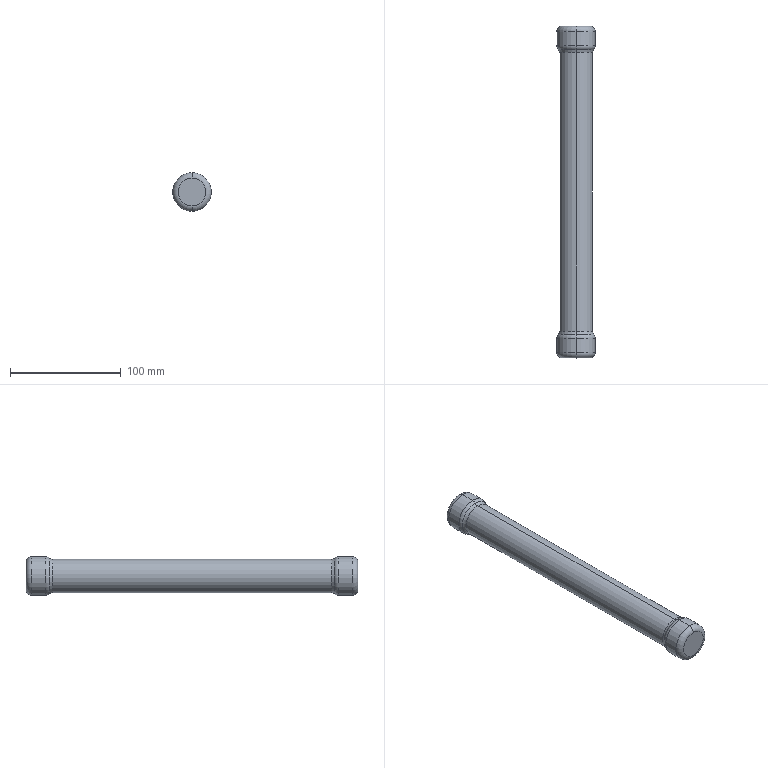Part | SolidWorks | features Fillet 3, Extrusion 1, ICE 1, MirrorPattern 1 | 1 solid | 20 faces | box 35 x 300 x 35 mm | volume 221656 mm3 | torus 12 | cylinder 6 | plane 2 | commonest cylinder face diameters 35 x4 30 x2
STEP:
#1=CARTESIAN_POINT('',(0.,132.284,17.5));
#2=VERTEX_POINT('',#1);
#3=CARTESIAN_POINT('',(0.,132.284,-17.5));
#4=VERTEX_POINT('',#3);
#5=CARTESIAN_POINT('',(0.,132.284,0.));
#6=DIRECTION('',(0.,1.,0.));
#7=DIRECTION('',(0.,0.,-1.));
#8=AXIS2_PLACEMENT_3D('',#5,#6,#7);
#9=CIRCLE('',#8,17.5);
#10=EDGE_CURVE('',#2,#4,#9,.T.);
#11=ORIENTED_EDGE('',*,*,#10,.F.);
#12=CARTESIAN_POINT('',(0.,128.977,16.25));
#13=VERTEX_POINT('',#12);
#14=CARTESIAN_POINT('',(0.,132.284,12.5));
#15=DIRECTION('',(1.,0.,0.));
#16=DIRECTION('',(0.,0.,-1.));
#17=AXIS2_PLACEMENT_3D('',#14,#15,#16);
#18=CIRCLE('',#17,5.);
#19=EDGE_CURVE('',#2,#13,#18,.T.);
#20=ORIENTED_EDGE('',*,*,#19,.T.);
#21=CARTESIAN_POINT('',(0.,128.977,-16.25));
#22=VERTEX_POINT('',#21);
#23=CARTESIAN_POINT('',(0.,128.977,0.));
#24=DIRECTION('',(0.,-1.,0.));
#25=DIRECTION('',(0.,0.,-1.));
#26=AXIS2_PLACEMENT_3D('',#23,#24,#25);
#27=CIRCLE('',#26,16.25);
#28=EDGE_CURVE('',#22,#13,#27,.T.);
#29=ORIENTED_EDGE('',*,*,#28,.F.);
#30=CARTESIAN_POINT('',(0.,132.284,-12.5));
#31=DIRECTION('',(-1.,0.,0.));
#32=DIRECTION('',(0.,0.,1.));
#33=AXIS2_PLACEMENT_3D('',#30,#31,#32);
#34=CIRCLE('',#33,5.);
#35=EDGE_CURVE('',#4,#22,#34,.T.);
#36=ORIENTED_EDGE('',*,*,#35,.F.);
#37=EDGE_LOOP('',(#11,#20,#29,#36));
#38=FACE_OUTER_BOUND('',#37,.T.);
#39=CARTESIAN_POINT('',(0.,132.284,0.));
#40=DIRECTION('',(0.,-1.,0.));
#41=DIRECTION('',(0.,0.,-1.));
#42=AXIS2_PLACEMENT_3D('',#39,#40,#41);
#43=TOROIDAL_SURFACE('',#42,12.5,5.);
#44=ADVANCED_FACE('',(#38),#43,.T.);
#45=CARTESIAN_POINT('',(0.,-128.977,16.25));
#46=VERTEX_POINT('',#45);
#47=CARTESIAN_POINT('',(0.,-128.977,-16.25));
#48=VERTEX_POINT('',#47);
#49=CARTESIAN_POINT('',(0.,-128.977,0.));
#50=DIRECTION('',(0.,1.,0.));
#51=DIRECTION('',(0.,0.,1.));
#52=AXIS2_PLACEMENT_3D('',#49,#50,#51);
#53=CIRCLE('',#52,16.25);
#54=EDGE_CURVE('',#46,#48,#53,.T.);
#55=ORIENTED_EDGE('',*,*,#54,.F.);
#56=CARTESIAN_POINT('',(0.,-132.284,17.5));
#57=VERTEX_POINT('',#56);
#58=CARTESIAN_POINT('',(0.,-132.284,12.5));
#59=DIRECTION('',(1.,0.,0.));
#60=DIRECTION('',(0.,0.,-1.));
#61=AXIS2_PLACEMENT_3D('',#58,#59,#60);
#62=CIRCLE('',#61,5.);
#63=EDGE_CURVE('',#46,#57,#62,.T.);
#64=ORIENTED_EDGE('',*,*,#63,.T.);
#65=CARTESIAN_POINT('',(0.,-132.284,-17.5));
#66=VERTEX_POINT('',#65);
#67=CARTESIAN_POINT('',(0.,-132.284,0.));
#68=DIRECTION('',(0.,-1.,0.));
#69=DIRECTION('',(0.,0.,-1.));
#70=AXIS2_PLACEMENT_3D('',#67,#68,#69);
#71=CIRCLE('',#70,17.5);
#72=EDGE_CURVE('',#66,#57,#71,.T.);
#73=ORIENTED_EDGE('',*,*,#72,.F.);
#74=CARTESIAN_POINT('',(0.,-132.284,-12.5));
#75=DIRECTION('',(-1.,0.,0.));
#76=DIRECTION('',(0.,0.,1.));
#77=AXIS2_PLACEMENT_3D('',#74,#75,#76);
#78=CIRCLE('',#77,5.);
#79=EDGE_CURVE('',#48,#66,#78,.T.);
#80=ORIENTED_EDGE('',*,*,#79,.F.);
#81=EDGE_LOOP('',(#55,#64,#73,#80));
#82=FACE_OUTER_BOUND('',#81,.T.);
#83=CARTESIAN_POINT('',(0.,-132.284,0.));
#84=DIRECTION('',(0.,-1.,0.));
#85=DIRECTION('',(0.,0.,-1.));
#86=AXIS2_PLACEMENT_3D('',#83,#84,#85);
#87=TOROIDAL_SURFACE('',#86,12.5,5.);
#88=ADVANCED_FACE('',(#82),#87,.T.);
#89=CARTESIAN_POINT('',(0.,-145.,17.5));
#90=VERTEX_POINT('',#89);
#91=CARTESIAN_POINT('',(0.,-145.,-17.5));
#92=VERTEX_POINT('',#91);
#93=CARTESIAN_POINT('',(0.,-145.,0.));
#94=DIRECTION('',(0.,1.,0.));
#95=DIRECTION('',(0.,0.,-1.));
#96=AXIS2_PLACEMENT_3D('',#93,#94,#95);
#97=CIRCLE('',#96,17.5);
#98=EDGE_CURVE('',#90,#92,#97,.T.);
#99=ORIENTED_EDGE('',*,*,#98,.F.);
#100=CARTESIAN_POINT('',(0.,-150.,12.5));
#101=VERTEX_POINT('',#100);
#102=CARTESIAN_POINT('',(0.,-145.,12.5));
#103=DIRECTION('',(1.,0.,0.));
#104=DIRECTION('',(0.,0.,-1.));
#105=AXIS2_PLACEMENT_3D('',#102,#103,#104);
#106=CIRCLE('',#105,5.);
#107=EDGE_CURVE('',#90,#101,#106,.T.);
#108=ORIENTED_EDGE('',*,*,#107,.T.);
#109=CARTESIAN_POINT('',(0.,-150.,-12.5));
#110=VERTEX_POINT('',#109);
#111=CARTESIAN_POINT('',(0.,-150.,0.));
#112=DIRECTION('',(0.,-1.,0.));
#113=DIRECTION('',(0.,0.,-1.));
#114=AXIS2_PLACEMENT_3D('',#111,#112,#113);
#115=CIRCLE('',#114,12.5);
#116=EDGE_CURVE('',#110,#101,#115,.T.);
#117=ORIENTED_EDGE('',*,*,#116,.F.);
#118=CARTESIAN_POINT('',(0.,-145.,-12.5));
#119=DIRECTION('',(-1.,0.,0.));
#120=DIRECTION('',(0.,0.,1.));
#121=AXIS2_PLACEMENT_3D('',#118,#119,#120);
#122=CIRCLE('',#121,5.);
#123=EDGE_CURVE('',#92,#110,#122,.T.);
#124=ORIENTED_EDGE('',*,*,#123,.F.);
#125=EDGE_LOOP('',(#99,#108,#117,#124));
#126=FACE_OUTER_BOUND('',#125,.T.);
#127=CARTESIAN_POINT('',(0.,-145.,0.));
#128=DIRECTION('',(0.,-1.,0.));
#129=DIRECTION('',(0.,0.,-1.));
#130=AXIS2_PLACEMENT_3D('',#127,#128,#129);
#131=TOROIDAL_SURFACE('',#130,12.5,5.);
#132=ADVANCED_FACE('',(#126),#131,.T.);
#133=CARTESIAN_POINT('',(0.,145.,-17.5));
#134=VERTEX_POINT('',#133);
#135=CARTESIAN_POINT('',(0.,145.,17.5));
#136=VERTEX_POINT('',#135);
#137=CARTESIAN_POINT('',(0.,145.,0.));
#138=DIRECTION('',(0.,-1.,0.));
#139=DIRECTION('',(0.,0.,1.));
#140=AXIS2_PLACEMENT_3D('',#137,#138,#139);
#141=CIRCLE('',#140,17.5);
#142=EDGE_CURVE('',#134,#136,#141,.T.);
#143=ORIENTED_EDGE('',*,*,#142,.F.);
#144=CARTESIAN_POINT('',(0.,150.,-12.5));
#145=VERTEX_POINT('',#144);
#146=CARTESIAN_POINT('',(0.,145.,-12.5));
#147=DIRECTION('',(1.,0.,0.));
#148=DIRECTION('',(0.,0.,-1.));
#149=AXIS2_PLACEMENT_3D('',#146,#147,#148);
#150=CIRCLE('',#149,5.);
#151=EDGE_CURVE('',#134,#145,#150,.T.);
#152=ORIENTED_EDGE('',*,*,#151,.T.);
#153=CARTESIAN_POINT('',(0.,150.,12.5));
#154=VERTEX_POINT('',#153);
#155=CARTESIAN_POINT('',(0.,150.,0.));
#156=DIRECTION('',(0.,1.,0.));
#157=DIRECTION('',(0.,0.,1.));
#158=AXIS2_PLACEMENT_3D('',#155,#156,#157);
#159=CIRCLE('',#158,12.5);
#160=EDGE_CURVE('',#154,#145,#159,.T.);
#161=ORIENTED_EDGE('',*,*,#160,.F.);
#162=CARTESIAN_POINT('',(0.,145.,12.5));
#163=DIRECTION('',(-1.,0.,0.));
#164=DIRECTION('',(0.,0.,1.));
#165=AXIS2_PLACEMENT_3D('',#162,#163,#164);
#166=CIRCLE('',#165,5.);
#167=EDGE_CURVE('',#136,#154,#166,.T.);
#168=ORIENTED_EDGE('',*,*,#167,.F.);
#169=EDGE_LOOP('',(#143,#152,#161,#168));
#170=FACE_OUTER_BOUND('',#169,.T.);
#171=CARTESIAN_POINT('',(0.,145.,0.));
#172=DIRECTION('',(0.,1.,0.));
#173=DIRECTION('',(0.,0.,1.));
#174=AXIS2_PLACEMENT_3D('',#171,#172,#173);
#175=TOROIDAL_SURFACE('',#174,12.5,5.);
#176=ADVANCED_FACE('',(#170),#175,.T.);
#177=CARTESIAN_POINT('',(0.,-128.977,0.));
#178=DIRECTION('',(0.,1.,0.));
#179=DIRECTION('',(0.,0.,1.));
#180=AXIS2_PLACEMENT_3D('',#177,#178,#179);
#181=CIRCLE('',#180,16.25);
#182=EDGE_CURVE('',#48,#46,#181,.T.);
#183=ORIENTED_EDGE('',*,*,#182,.T.);
#184=CARTESIAN_POINT('',(0.,-125.67,15.));
#185=VERTEX_POINT('',#184);
#186=CARTESIAN_POINT('',(0.,-125.67,20.));
#187=DIRECTION('',(1.,0.,0.));
#188=DIRECTION('',(0.,0.,-1.));
#189=AXIS2_PLACEMENT_3D('',#186,#187,#188);
#190=CIRCLE('',#189,5.);
#191=EDGE_CURVE('',#46,#185,#190,.T.);
#192=ORIENTED_EDGE('',*,*,#191,.T.);
#193=CARTESIAN_POINT('',(0.,-125.67,-15.));
#194=VERTEX_POINT('',#193);
#195=CARTESIAN_POINT('',(0.,-125.67,0.));
#196=DIRECTION('',(0.,1.,0.));
#197=DIRECTION('',(0.,0.,-1.));
#198=AXIS2_PLACEMENT_3D('',#195,#196,#197);
#199=CIRCLE('',#198,15.);
#200=EDGE_CURVE('',#194,#185,#199,.T.);
#201=ORIENTED_EDGE('',*,*,#200,.F.);
#202=CARTESIAN_POINT('',(0.,-125.67,-20.));
#203=DIRECTION('',(-1.,0.,0.));
#204=DIRECTION('',(0.,0.,1.));
#205=AXIS2_PLACEMENT_3D('',#202,#203,#204);
#206=CIRCLE('',#205,5.);
#207=EDGE_CURVE('',#48,#194,#206,.T.);
#208=ORIENTED_EDGE('',*,*,#207,.F.);
#209=EDGE_LOOP('',(#183,#192,#201,#208));
#210=FACE_OUTER_BOUND('',#209,.T.);
#211=CARTESIAN_POINT('',(0.,-125.67,0.));
#212=DIRECTION('',(0.,-1.,0.));
#213=DIRECTION('',(0.,0.,-1.));
#214=AXIS2_PLACEMENT_3D('',#211,#212,#213);
#215=TOROIDAL_SURFACE('',#214,20.,5.);
#216=ADVANCED_FACE('',(#210),#215,.F.);
#217=CARTESIAN_POINT('',(0.,128.977,0.));
#218=DIRECTION('',(0.,-1.,0.));
#219=DIRECTION('',(0.,0.,-1.));
#220=AXIS2_PLACEMENT_3D('',#217,#218,#219);
#221=CIRCLE('',#220,16.25);
#222=EDGE_CURVE('',#13,#22,#221,.T.);
#223=ORIENTED_EDGE('',*,*,#222,.T.);
#224=CARTESIAN_POINT('',(0.,125.67,-15.));
#225=VERTEX_POINT('',#224);
#226=CARTESIAN_POINT('',(0.,125.67,-20.));
#227=DIRECTION('',(1.,0.,0.));
#228=DIRECTION('',(0.,0.,-1.));
#229=AXIS2_PLACEMENT_3D('',#226,#227,#228);
#230=CIRCLE('',#229,5.);
#231=EDGE_CURVE('',#22,#225,#230,.T.);
#232=ORIENTED_EDGE('',*,*,#231,.T.);
#233=CARTESIAN_POINT('',(0.,125.67,15.));
#234=VERTEX_POINT('',#233);
#235=CARTESIAN_POINT('',(0.,125.67,0.));
#236=DIRECTION('',(0.,-1.,0.));
#237=DIRECTION('',(0.,0.,1.));
#238=AXIS2_PLACEMENT_3D('',#235,#236,#237);
#239=CIRCLE('',#238,15.);
#240=EDGE_CURVE('',#234,#225,#239,.T.);
#241=ORIENTED_EDGE('',*,*,#240,.F.);
#242=CARTESIAN_POINT('',(0.,125.67,20.));
#243=DIRECTION('',(-1.,0.,0.));
#244=DIRECTION('',(0.,0.,1.));
#245=AXIS2_PLACEMENT_3D('',#242,#243,#244);
#246=CIRCLE('',#245,5.);
#247=EDGE_CURVE('',#13,#234,#246,.T.);
#248=ORIENTED_EDGE('',*,*,#247,.F.);
#249=EDGE_LOOP('',(#223,#232,#241,#248));
#250=FACE_OUTER_BOUND('',#249,.T.);
#251=CARTESIAN_POINT('',(0.,125.67,0.));
#252=DIRECTION('',(0.,1.,0.));
#253=DIRECTION('',(0.,0.,1.));
#254=AXIS2_PLACEMENT_3D('',#251,#252,#253);
#255=TOROIDAL_SURFACE('',#254,20.,5.);
#256=ADVANCED_FACE('',(#250),#255,.F.);
#257=ORIENTED_EDGE('',*,*,#98,.T.);
#258=CARTESIAN_POINT('',(0.,-150.,-17.5));
#259=DIRECTION('',(0.,1.,0.));
#260=VECTOR('',#259,1000.);
#261=LINE('',#258,#260);
#262=EDGE_CURVE('',#92,#66,#261,.T.);
#263=ORIENTED_EDGE('',*,*,#262,.T.);
#264=ORIENTED_EDGE('',*,*,#72,.T.);
#265=CARTESIAN_POINT('',(0.,-150.,17.5));
#266=DIRECTION('',(0.,1.,0.));
#267=VECTOR('',#266,1000.);
#268=LINE('',#265,#267);
#269=EDGE_CURVE('',#90,#57,#268,.T.);
#270=ORIENTED_EDGE('',*,*,#269,.F.);
#271=EDGE_LOOP('',(#257,#263,#264,#270));
#272=FACE_OUTER_BOUND('',#271,.T.);
#273=CARTESIAN_POINT('',(0.,-150.,0.));
#274=DIRECTION('',(0.,1.,0.));
#275=DIRECTION('',(0.,0.,1.));
#276=AXIS2_PLACEMENT_3D('',#273,#274,#275);
#277=CYLINDRICAL_SURFACE('',#276,17.5);
#278=ADVANCED_FACE('',(#272),#277,.T.);
#279=ORIENTED_EDGE('',*,*,#142,.T.);
#280=CARTESIAN_POINT('',(0.,150.,17.5));
#281=DIRECTION('',(0.,-1.,0.));
#282=VECTOR('',#281,1000.);
#283=LINE('',#280,#282);
#284=EDGE_CURVE('',#136,#2,#283,.T.);
#285=ORIENTED_EDGE('',*,*,#284,.T.);
#286=ORIENTED_EDGE('',*,*,#10,.T.);
#287=CARTESIAN_POINT('',(0.,150.,-17.5));
#288=DIRECTION('',(0.,-1.,0.));
#289=VECTOR('',#288,1000.);
#290=LINE('',#287,#289);
#291=EDGE_CURVE('',#134,#4,#290,.T.);
#292=ORIENTED_EDGE('',*,*,#291,.F.);
#293=EDGE_LOOP('',(#279,#285,#286,#292));
#294=FACE_OUTER_BOUND('',#293,.T.);
#295=CARTESIAN_POINT('',(0.,150.,0.));
#296=DIRECTION('',(0.,-1.,0.));
#297=DIRECTION('',(0.,0.,-1.));
#298=AXIS2_PLACEMENT_3D('',#295,#296,#297);
#299=CYLINDRICAL_SURFACE('',#298,17.5);
#300=ADVANCED_FACE('',(#294),#299,.T.);
#301=CARTESIAN_POINT('',(0.,125.67,0.));
#302=DIRECTION('',(0.,-1.,0.));
#303=DIRECTION('',(0.,0.,1.));
#304=AXIS2_PLACEMENT_3D('',#301,#302,#303);
#305=CIRCLE('',#304,15.);
#306=EDGE_CURVE('',#225,#234,#305,.T.);
#307=ORIENTED_EDGE('',*,*,#306,.T.);
#308=CARTESIAN_POINT('',(0.,140.,15.));
#309=DIRECTION('',(0.,-1.,0.));
#310=VECTOR('',#309,1000.);
#311=LINE('',#308,#310);
#312=EDGE_CURVE('',#234,#185,#311,.T.);
#313=ORIENTED_EDGE('',*,*,#312,.T.);
#314=CARTESIAN_POINT('',(0.,-125.67,0.));
#315=DIRECTION('',(0.,1.,0.));
#316=DIRECTION('',(0.,0.,-1.));
#317=AXIS2_PLACEMENT_3D('',#314,#315,#316);
#318=CIRCLE('',#317,15.);
#319=EDGE_CURVE('',#185,#194,#318,.T.);
#320=ORIENTED_EDGE('',*,*,#319,.T.);
#321=CARTESIAN_POINT('',(0.,140.,-15.));
#322=DIRECTION('',(0.,-1.,0.));
#323=VECTOR('',#322,1000.);
#324=LINE('',#321,#323);
#325=EDGE_CURVE('',#225,#194,#324,.T.);
#326=ORIENTED_EDGE('',*,*,#325,.F.);
#327=EDGE_LOOP('',(#307,#313,#320,#326));
#328=FACE_OUTER_BOUND('',#327,.T.);
#329=CARTESIAN_POINT('',(0.,140.,0.));
#330=DIRECTION('',(0.,-1.,0.));
#331=DIRECTION('',(0.,0.,-1.));
#332=AXIS2_PLACEMENT_3D('',#329,#330,#331);
#333=CYLINDRICAL_SURFACE('',#332,15.);
#334=ADVANCED_FACE('',(#328),#333,.T.);
#335=ORIENTED_EDGE('',*,*,#312,.F.);
#336=ORIENTED_EDGE('',*,*,#240,.T.);
#337=ORIENTED_EDGE('',*,*,#325,.T.);
#338=ORIENTED_EDGE('',*,*,#200,.T.);
#339=EDGE_LOOP('',(#335,#336,#337,#338));
#340=FACE_OUTER_BOUND('',#339,.T.);
#341=CARTESIAN_POINT('',(0.,140.,0.));
#342=DIRECTION('',(0.,-1.,0.));
#343=DIRECTION('',(0.,0.,-1.));
#344=AXIS2_PLACEMENT_3D('',#341,#342,#343);
#345=CYLINDRICAL_SURFACE('',#344,15.);
#346=ADVANCED_FACE('',(#340),#345,.T.);
#347=ORIENTED_EDGE('',*,*,#284,.F.);
#348=CARTESIAN_POINT('',(0.,145.,0.));
#349=DIRECTION('',(0.,-1.,0.));
#350=DIRECTION('',(0.,0.,1.));
#351=AXIS2_PLACEMENT_3D('',#348,#349,#350);
#352=CIRCLE('',#351,17.5);
#353=EDGE_CURVE('',#136,#134,#352,.T.);
#354=ORIENTED_EDGE('',*,*,#353,.T.);
#355=ORIENTED_EDGE('',*,*,#291,.T.);
#356=CARTESIAN_POINT('',(0.,132.284,0.));
#357=DIRECTION('',(0.,1.,0.));
#358=DIRECTION('',(0.,0.,-1.));
#359=AXIS2_PLACEMENT_3D('',#356,#357,#358);
#360=CIRCLE('',#359,17.5);
#361=EDGE_CURVE('',#4,#2,#360,.T.);
#362=ORIENTED_EDGE('',*,*,#361,.T.);
#363=EDGE_LOOP('',(#347,#354,#355,#362));
#364=FACE_OUTER_BOUND('',#363,.T.);
#365=CARTESIAN_POINT('',(0.,150.,0.));
#366=DIRECTION('',(0.,-1.,0.));
#367=DIRECTION('',(0.,0.,-1.));
#368=AXIS2_PLACEMENT_3D('',#365,#366,#367);
#369=CYLINDRICAL_SURFACE('',#368,17.5);
#370=ADVANCED_FACE('',(#364),#369,.T.);
#371=ORIENTED_EDGE('',*,*,#160,.T.);
#372=CARTESIAN_POINT('',(0.,150.,0.));
#373=DIRECTION('',(0.,1.,0.));
#374=DIRECTION('',(0.,0.,1.));
#375=AXIS2_PLACEMENT_3D('',#372,#373,#374);
#376=CIRCLE('',#375,12.5);
#377=EDGE_CURVE('',#145,#154,#376,.T.);
#378=ORIENTED_EDGE('',*,*,#377,.T.);
#379=EDGE_LOOP('',(#371,#378));
#380=FACE_OUTER_BOUND('',#379,.T.);
#381=CARTESIAN_POINT('',(0.,150.,0.));
#382=DIRECTION('',(0.,1.,0.));
#383=DIRECTION('',(0.,0.,1.));
#384=AXIS2_PLACEMENT_3D('',#381,#382,#383);
#385=PLANE('',#384);
#386=ADVANCED_FACE('',(#380),#385,.T.);
#387=ORIENTED_EDGE('',*,*,#262,.F.);
#388=CARTESIAN_POINT('',(0.,-145.,0.));
#389=DIRECTION('',(0.,1.,0.));
#390=DIRECTION('',(0.,0.,-1.));
#391=AXIS2_PLACEMENT_3D('',#388,#389,#390);
#392=CIRCLE('',#391,17.5);
#393=EDGE_CURVE('',#92,#90,#392,.T.);
#394=ORIENTED_EDGE('',*,*,#393,.T.);
#395=ORIENTED_EDGE('',*,*,#269,.T.);
#396=CARTESIAN_POINT('',(0.,-132.284,0.));
#397=DIRECTION('',(0.,-1.,0.));
#398=DIRECTION('',(0.,0.,-1.));
#399=AXIS2_PLACEMENT_3D('',#396,#397,#398);
#400=CIRCLE('',#399,17.5);
#401=EDGE_CURVE('',#57,#66,#400,.T.);
#402=ORIENTED_EDGE('',*,*,#401,.T.);
#403=EDGE_LOOP('',(#387,#394,#395,#402));
#404=FACE_OUTER_BOUND('',#403,.T.);
#405=CARTESIAN_POINT('',(0.,-150.,0.));
#406=DIRECTION('',(0.,1.,0.));
#407=DIRECTION('',(0.,0.,1.));
#408=AXIS2_PLACEMENT_3D('',#405,#406,#407);
#409=CYLINDRICAL_SURFACE('',#408,17.5);
#410=ADVANCED_FACE('',(#404),#409,.T.);
#411=ORIENTED_EDGE('',*,*,#116,.T.);
#412=CARTESIAN_POINT('',(0.,-150.,0.));
#413=DIRECTION('',(0.,-1.,0.));
#414=DIRECTION('',(0.,0.,-1.));
#415=AXIS2_PLACEMENT_3D('',#412,#413,#414);
#416=CIRCLE('',#415,12.5);
#417=EDGE_CURVE('',#101,#110,#416,.T.);
#418=ORIENTED_EDGE('',*,*,#417,.T.);
#419=EDGE_LOOP('',(#411,#418));
#420=FACE_OUTER_BOUND('',#419,.T.);
#421=CARTESIAN_POINT('',(0.,-150.,0.));
#422=DIRECTION('',(0.,-1.,0.));
#423=DIRECTION('',(0.,0.,1.));
#424=AXIS2_PLACEMENT_3D('',#421,#422,#423);
#425=PLANE('',#424);
#426=ADVANCED_FACE('',(#420),#425,.T.);
#427=ORIENTED_EDGE('',*,*,#231,.F.);
#428=ORIENTED_EDGE('',*,*,#28,.T.);
#429=ORIENTED_EDGE('',*,*,#247,.T.);
#430=ORIENTED_EDGE('',*,*,#306,.F.);
#431=EDGE_LOOP('',(#427,#428,#429,#430));
#432=FACE_OUTER_BOUND('',#431,.T.);
#433=CARTESIAN_POINT('',(0.,125.67,0.));
#434=DIRECTION('',(0.,1.,0.));
#435=DIRECTION('',(0.,0.,1.));
#436=AXIS2_PLACEMENT_3D('',#433,#434,#435);
#437=TOROIDAL_SURFACE('',#436,20.,5.);
#438=ADVANCED_FACE('',(#432),#437,.F.);
#439=ORIENTED_EDGE('',*,*,#191,.F.);
#440=ORIENTED_EDGE('',*,*,#54,.T.);
#441=ORIENTED_EDGE('',*,*,#207,.T.);
#442=ORIENTED_EDGE('',*,*,#319,.F.);
#443=EDGE_LOOP('',(#439,#440,#441,#442));
#444=FACE_OUTER_BOUND('',#443,.T.);
#445=CARTESIAN_POINT('',(0.,-125.67,0.));
#446=DIRECTION('',(0.,-1.,0.));
#447=DIRECTION('',(0.,0.,-1.));
#448=AXIS2_PLACEMENT_3D('',#445,#446,#447);
#449=TOROIDAL_SURFACE('',#448,20.,5.);
#450=ADVANCED_FACE('',(#444),#449,.F.);
#451=ORIENTED_EDGE('',*,*,#151,.F.);
#452=ORIENTED_EDGE('',*,*,#353,.F.);
#453=ORIENTED_EDGE('',*,*,#167,.T.);
#454=ORIENTED_EDGE('',*,*,#377,.F.);
#455=EDGE_LOOP('',(#451,#452,#453,#454));
#456=FACE_OUTER_BOUND('',#455,.T.);
#457=CARTESIAN_POINT('',(0.,145.,0.));
#458=DIRECTION('',(0.,1.,0.));
#459=DIRECTION('',(0.,0.,1.));
#460=AXIS2_PLACEMENT_3D('',#457,#458,#459);
#461=TOROIDAL_SURFACE('',#460,12.5,5.);
#462=ADVANCED_FACE('',(#456),#461,.T.);
#463=ORIENTED_EDGE('',*,*,#107,.F.);
#464=ORIENTED_EDGE('',*,*,#393,.F.);
#465=ORIENTED_EDGE('',*,*,#123,.T.);
#466=ORIENTED_EDGE('',*,*,#417,.F.);
#467=EDGE_LOOP('',(#463,#464,#465,#466));
#468=FACE_OUTER_BOUND('',#467,.T.);
#469=CARTESIAN_POINT('',(0.,-145.,0.));
#470=DIRECTION('',(0.,-1.,0.));
#471=DIRECTION('',(0.,0.,-1.));
#472=AXIS2_PLACEMENT_3D('',#469,#470,#471);
#473=TOROIDAL_SURFACE('',#472,12.5,5.);
#474=ADVANCED_FACE('',(#468),#473,.T.);
#475=ORIENTED_EDGE('',*,*,#63,.F.);
#476=ORIENTED_EDGE('',*,*,#182,.F.);
#477=ORIENTED_EDGE('',*,*,#79,.T.);
#478=ORIENTED_EDGE('',*,*,#401,.F.);
#479=EDGE_LOOP('',(#475,#476,#477,#478));
#480=FACE_OUTER_BOUND('',#479,.T.);
#481=CARTESIAN_POINT('',(0.,-132.284,0.));
#482=DIRECTION('',(0.,-1.,0.));
#483=DIRECTION('',(0.,0.,-1.));
#484=AXIS2_PLACEMENT_3D('',#481,#482,#483);
#485=TOROIDAL_SURFACE('',#484,12.5,5.);
#486=ADVANCED_FACE('',(#480),#485,.T.);
#487=ORIENTED_EDGE('',*,*,#19,.F.);
#488=ORIENTED_EDGE('',*,*,#361,.F.);
#489=ORIENTED_EDGE('',*,*,#35,.T.);
#490=ORIENTED_EDGE('',*,*,#222,.F.);
#491=EDGE_LOOP('',(#487,#488,#489,#490));
#492=FACE_OUTER_BOUND('',#491,.T.);
#493=CARTESIAN_POINT('',(0.,132.284,0.));
#494=DIRECTION('',(0.,-1.,0.));
#495=DIRECTION('',(0.,0.,-1.));
#496=AXIS2_PLACEMENT_3D('',#493,#494,#495);
#497=TOROIDAL_SURFACE('',#496,12.5,5.);
#498=ADVANCED_FACE('',(#492),#497,.T.);
#499=CLOSED_SHELL('',(#44,#88,#132,#176,#216,#256,#278,#300,#334,#346,#370,#386,#410,#426,#438,#450,#462,#474,#486,#498));
#500=MANIFOLD_SOLID_BREP('',#499);
#501=CARTESIAN_POINT('',(0.,0.,0.));
#502=DIRECTION('',(0.,0.,1.));
#503=DIRECTION('',(1.,0.,0.));
#504=AXIS2_PLACEMENT_3D('',#501,#502,#503);
#505=(LENGTH_UNIT()NAMED_UNIT(*)SI_UNIT(.MILLI.,.METRE.));
#506=UNCERTAINTY_MEASURE_WITH_UNIT(LENGTH_MEASURE(0.00001),#505,'','');
#507=(NAMED_UNIT(*)PLANE_ANGLE_UNIT()SI_UNIT($,.RADIAN.));
#508=(NAMED_UNIT(*)SI_UNIT($,.STERADIAN.)SOLID_ANGLE_UNIT());
#509=(GEOMETRIC_REPRESENTATION_CONTEXT(3)GLOBAL_UNCERTAINTY_ASSIGNED_CONTEXT((#506))GLOBAL_UNIT_ASSIGNED_CONTEXT((#505,#507,#508))REPRESENTATION_CONTEXT('',''));
#510=ADVANCED_BREP_SHAPE_REPRESENTATION('',(#500,#504),#509);